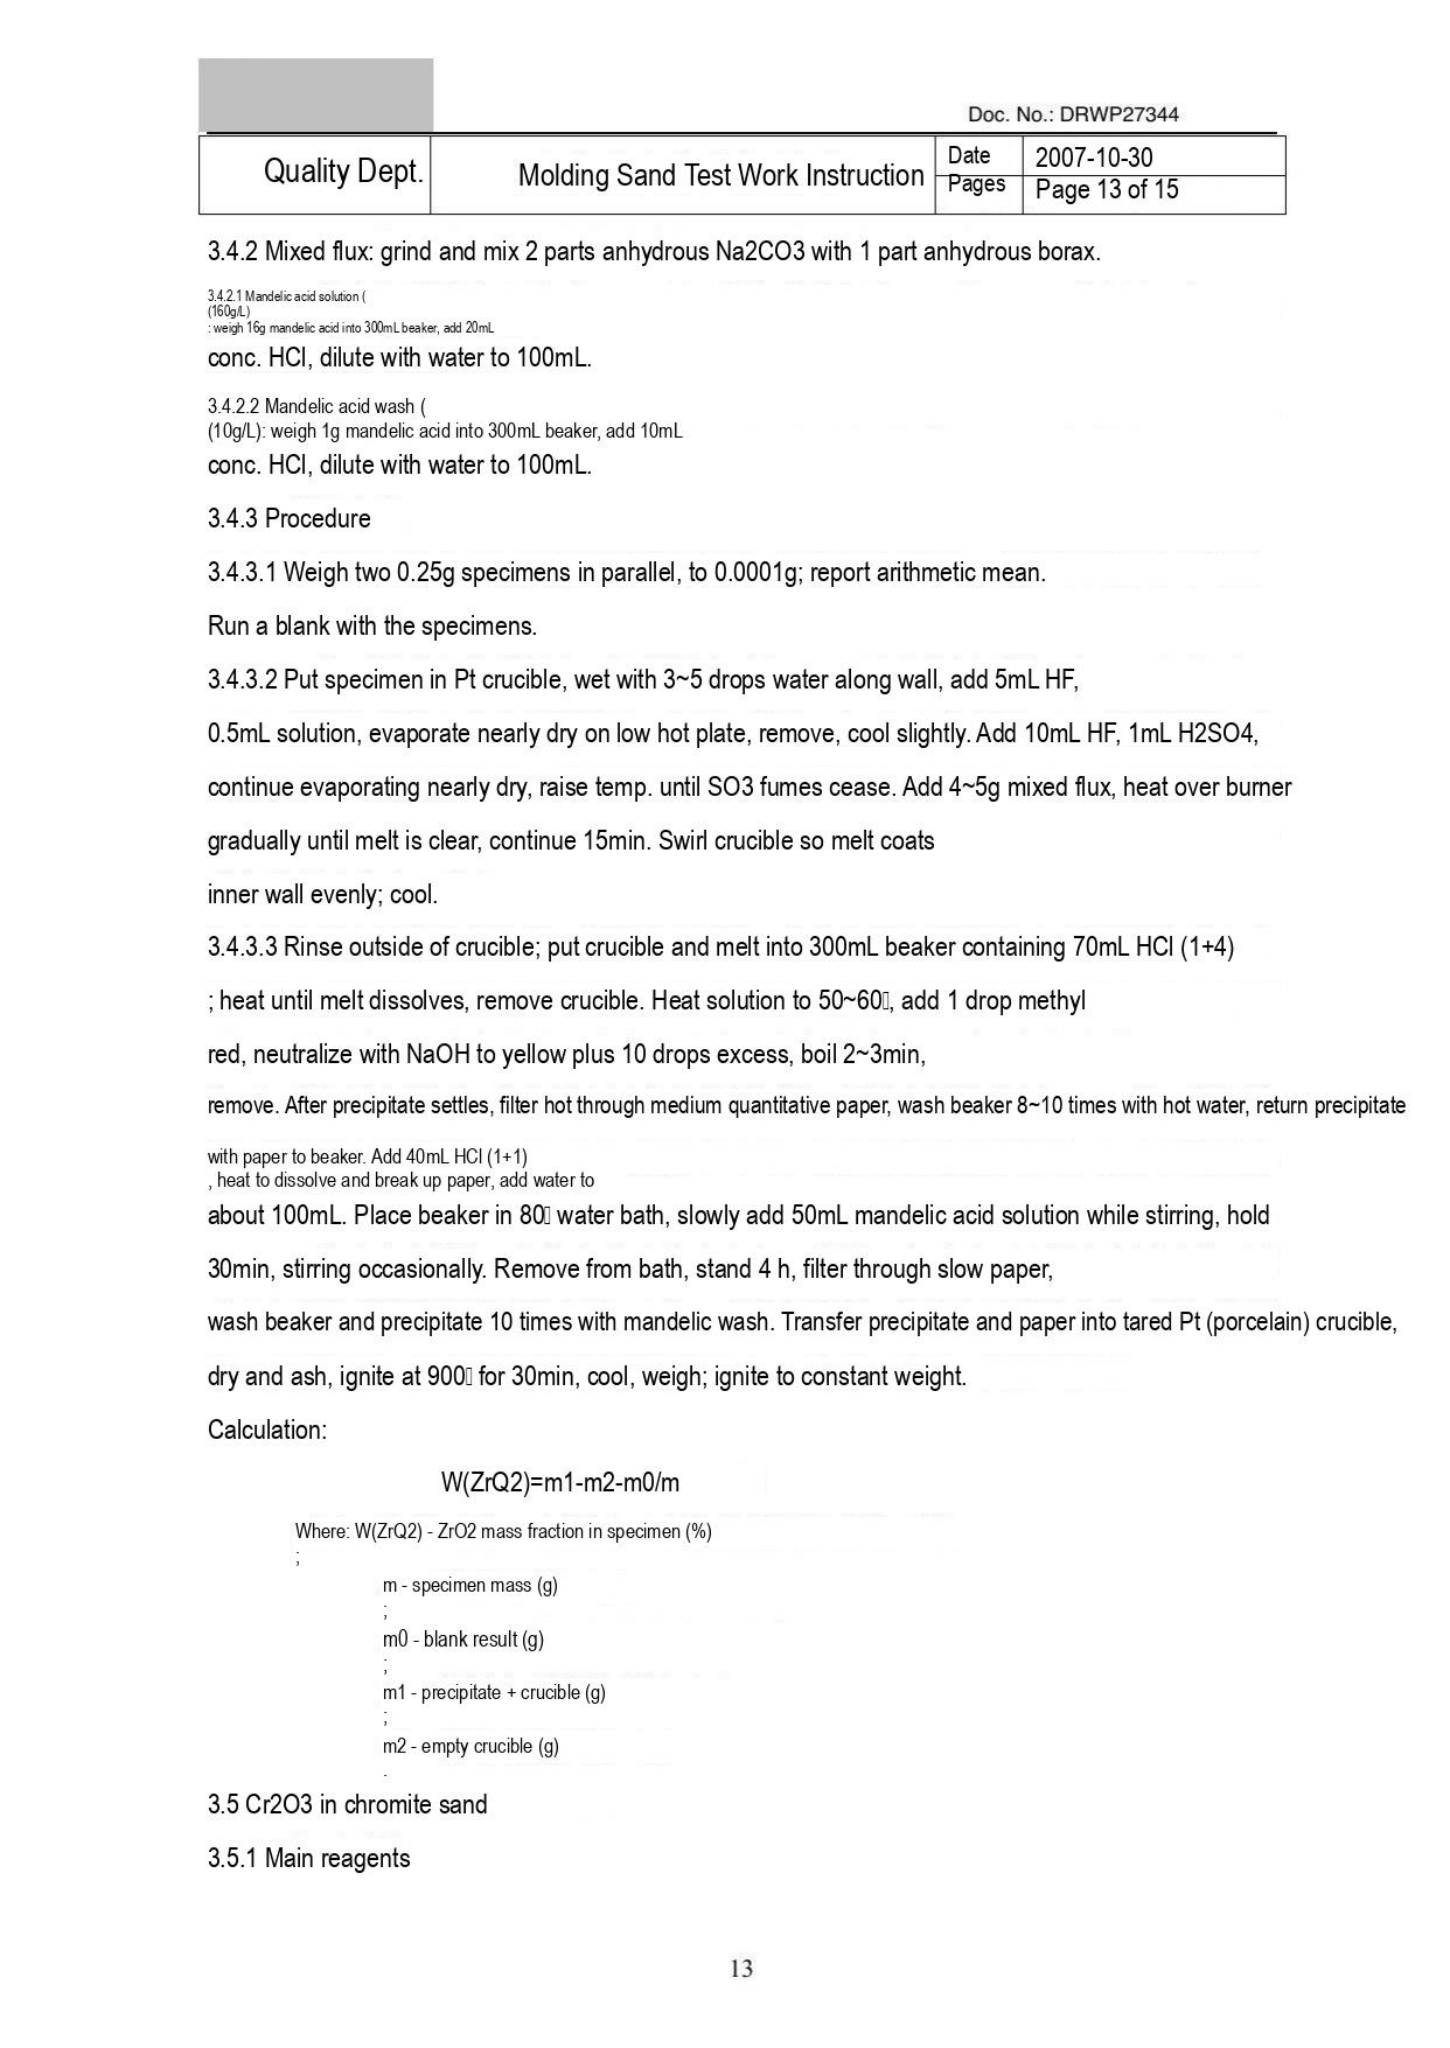Doc. No.: DRWP27344

| Quality Dept. | Molding Sand Test Work Instruction | Date | 2007-10-30 |
|---|---|---|---|
| | | Pages | Page 13 of 15 |

3.4.2 Mixed flux: grind and mix 2 parts anhydrous Na2CO3 with 1 part anhydrous borax.

3.4.2.1 Mandelic acid solution (
(160g/L)
: weigh 16g mandelic acid into 300mL beaker, add 20mL
conc. HCl, dilute with water to 100mL.

3.4.2.2 Mandelic acid wash (
(10g/L): weigh 1g mandelic acid into 300mL beaker, add 10mL
conc. HCl, dilute with water to 100mL.

3.4.3 Procedure

3.4.3.1 Weigh two 0.25g specimens in parallel, to 0.0001g; report arithmetic mean.

Run a blank with the specimens.

3.4.3.2 Put specimen in Pt crucible, wet with 3~5 drops water along wall, add 5mL HF,

0.5mL solution, evaporate nearly dry on low hot plate, remove, cool slightly. Add 10mL HF, 1mL H2SO4,

continue evaporating nearly dry, raise temp. until SO3 fumes cease. Add 4~5g mixed flux, heat over burner

gradually until melt is clear, continue 15min. Swirl crucible so melt coats

inner wall evenly; cool.

3.4.3.3 Rinse outside of crucible; put crucible and melt into 300mL beaker containing 70mL HCl (1+4)

; heat until melt dissolves, remove crucible. Heat solution to 50~60, add 1 drop methyl

red, neutralize with NaOH to yellow plus 10 drops excess, boil 2~3min,

remove. After precipitate settles, filter hot through medium quantitative paper, wash beaker 8~10 times with hot water, return precipitate

with paper to beaker. Add 40mL HCl (1+1)
, heat to dissolve and break up paper, add water to

about 100mL. Place beaker in 80 water bath, slowly add 50mL mandelic acid solution while stirring, hold

30min, stirring occasionally. Remove from bath, stand 4 h, filter through slow paper,

wash beaker and precipitate 10 times with mandelic wash. Transfer precipitate and paper into tared Pt (porcelain) crucible,

dry and ash, ignite at 900 for 30min, cool, weigh; ignite to constant weight.

Calculation:

W(ZrQ2)=m1-m2-m0/m

Where: W(ZrQ2) - ZrO2 mass fraction in specimen (%)
;

m - specimen mass (g)
;

m0 - blank result (g)
;

m1 - precipitate + crucible (g)
;

m2 - empty crucible (g)
.

3.5 Cr2O3 in chromite sand

3.5.1 Main reagents

13
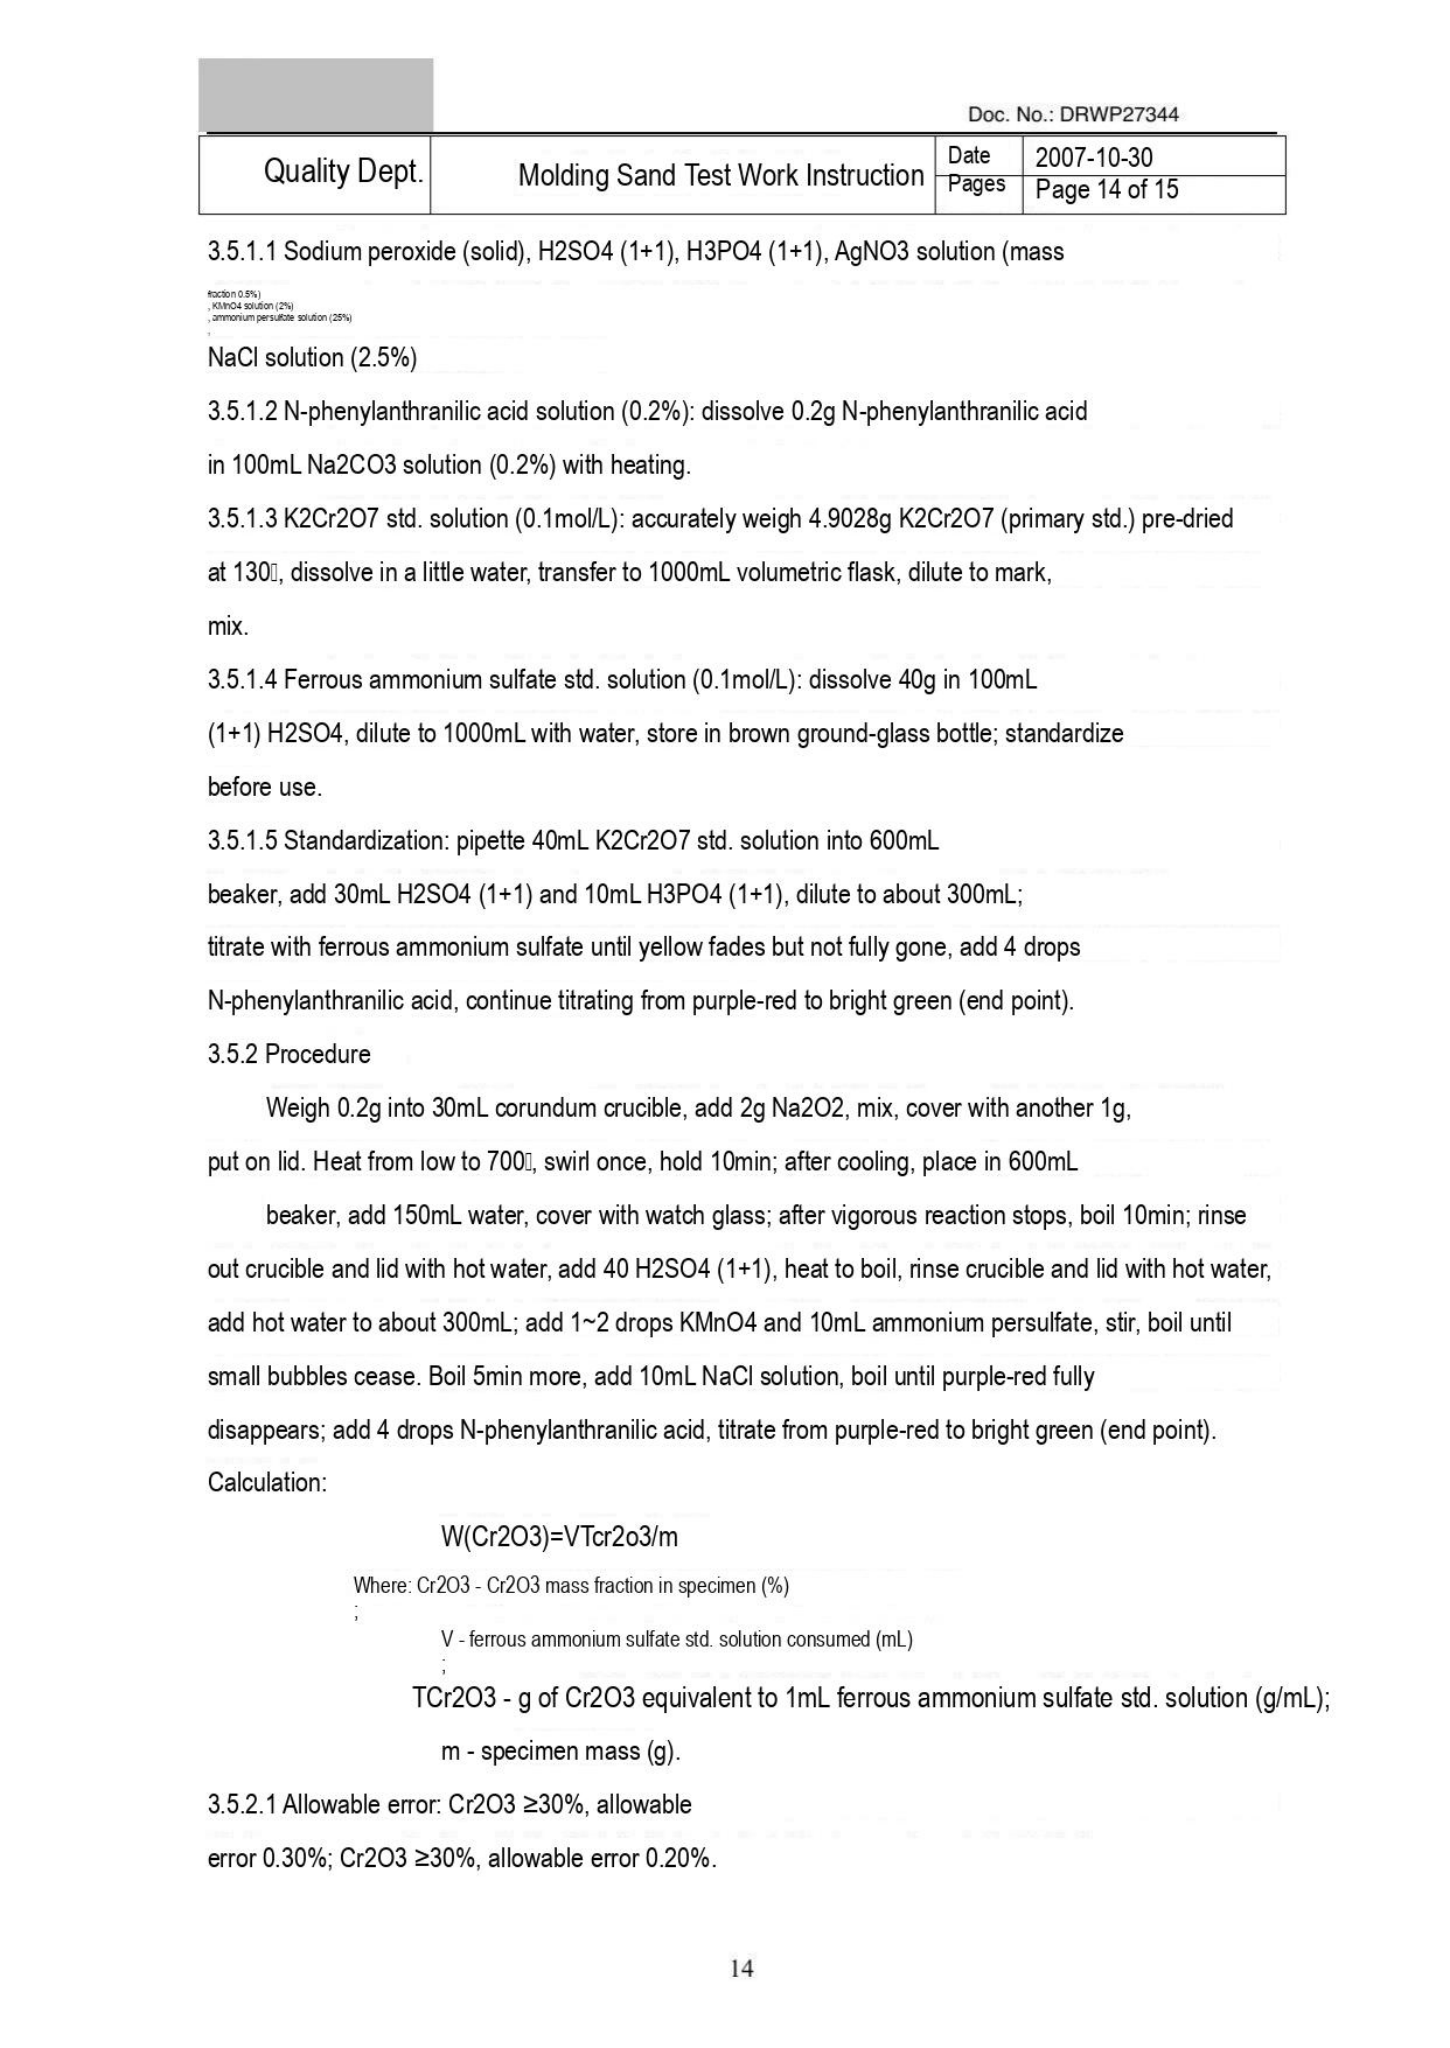Doc. No.: DRWP27344

| Quality Dept. | Molding Sand Test Work Instruction | Date | 2007-10-30 |
|---|---|---|---|
| | | Pages | Page 14 of 15 |

3.5.1.1 Sodium peroxide (solid), H2SO4 (1+1), H3PO4 (1+1), AgNO3 solution (mass

fraction 0.5%)
, KMnO4 solution (2%)
, ammonium persulfate solution (25%)
,
NaCl solution (2.5%)

3.5.1.2 N-phenylanthranilic acid solution (0.2%): dissolve 0.2g N-phenylanthranilic acid in 100mL Na2CO3 solution (0.2%) with heating.

3.5.1.3 K2Cr2O7 std. solution (0.1mol/L): accurately weigh 4.9028g K2Cr2O7 (primary std.) pre-dried at 130, dissolve in a little water, transfer to 1000mL volumetric flask, dilute to mark, mix.

3.5.1.4 Ferrous ammonium sulfate std. solution (0.1mol/L): dissolve 40g in 100mL (1+1) H2SO4, dilute to 1000mL with water, store in brown ground-glass bottle; standardize before use.

3.5.1.5 Standardization: pipette 40mL K2Cr2O7 std. solution into 600mL beaker, add 30mL H2SO4 (1+1) and 10mL H3PO4 (1+1), dilute to about 300mL; titrate with ferrous ammonium sulfate until yellow fades but not fully gone, add 4 drops N-phenylanthranilic acid, continue titrating from purple-red to bright green (end point).

3.5.2 Procedure

Weigh 0.2g into 30mL corundum crucible, add 2g Na2O2, mix, cover with another 1g, put on lid. Heat from low to 700, swirl once, hold 10min; after cooling, place in 600mL

beaker, add 150mL water, cover with watch glass; after vigorous reaction stops, boil 10min; rinse out crucible and lid with hot water, add 40 H2SO4 (1+1), heat to boil, rinse crucible and lid with hot water, add hot water to about 300mL; add 1~2 drops KMnO4 and 10mL ammonium persulfate, stir, boil until small bubbles cease. Boil 5min more, add 10mL NaCl solution, boil until purple-red fully disappears; add 4 drops N-phenylanthranilic acid, titrate from purple-red to bright green (end point).

Calculation:

W(Cr2O3)=VTcr2o3/m

Where: Cr2O3 - Cr2O3 mass fraction in specimen (%)
;
V - ferrous ammonium sulfate std. solution consumed (mL)
;
TCr2O3 - g of Cr2O3 equivalent to 1mL ferrous ammonium sulfate std. solution (g/mL);

m - specimen mass (g).

3.5.2.1 Allowable error: Cr2O3 ≥30%, allowable error 0.30%; Cr2O3 ≥30%, allowable error 0.20%.

14
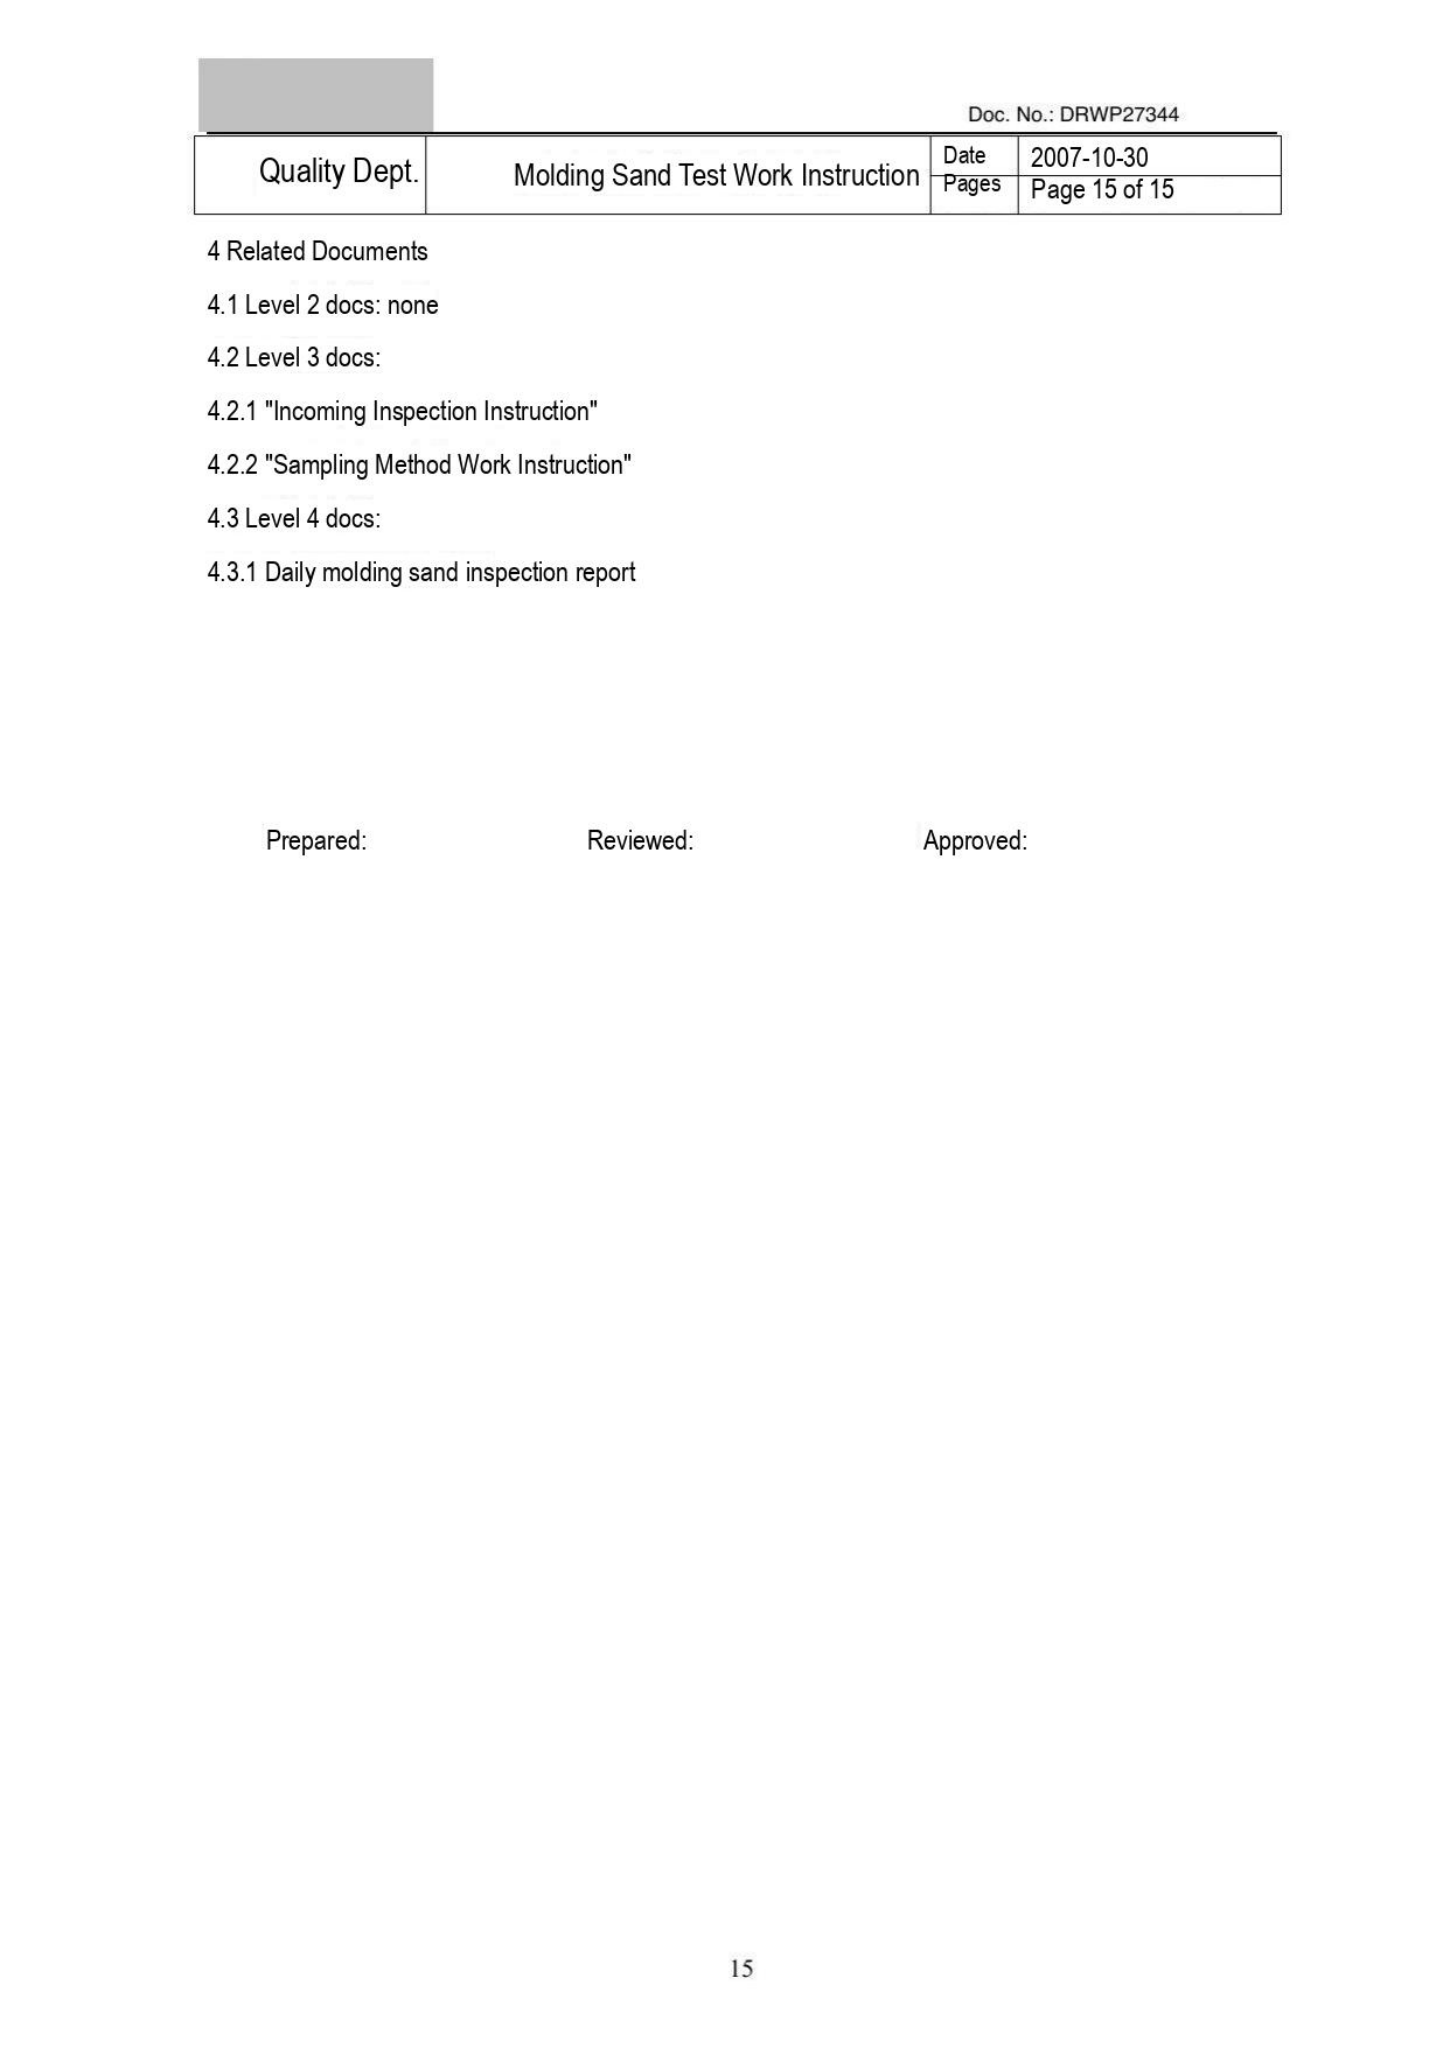Doc. No.: DRWP27344

| Quality Dept. | Molding Sand Test Work Instruction | Date | 2007-10-30 |
|---|---|---|---|
| | | Pages | Page 15 of 15 |

4 Related Documents

4.1 Level 2 docs: none

4.2 Level 3 docs:

4.2.1 "Incoming Inspection Instruction"

4.2.2 "Sampling Method Work Instruction"

4.3 Level 4 docs:

4.3.1 Daily molding sand inspection report

Prepared: Reviewed: Approved:

15